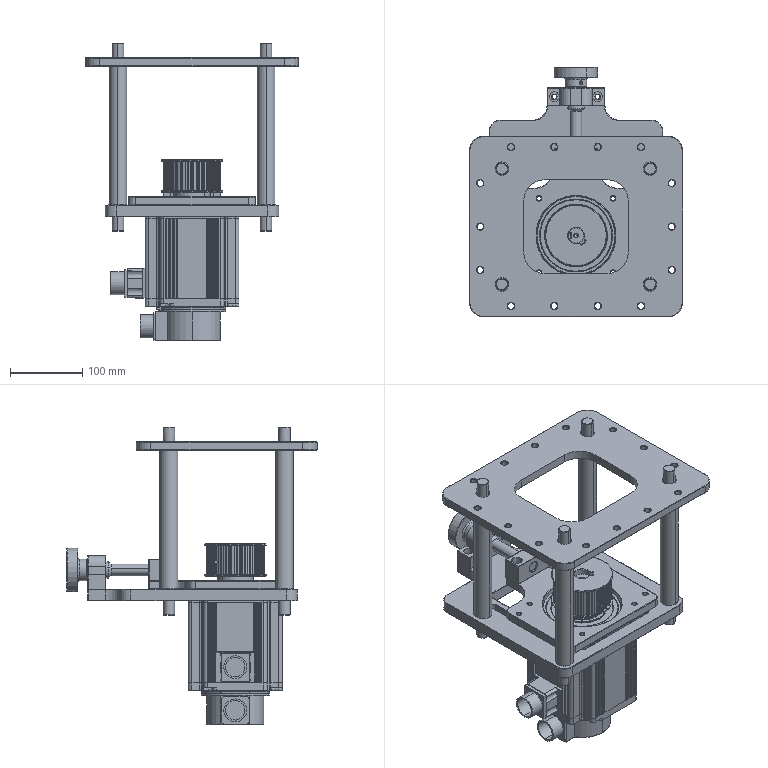Part | SolidWorks | 14 solids | 1575 faces | box 295 x 346 x 412 mm | volume 272069 mm3 | plane 568 | cylinder 509 | cone 428 | spline 55 | torus 14 | sphere 1 | commonest cylinder face diameters 2 x156 9 x40 80.12 x35 18 x32 77.12 x32 6.5 x24